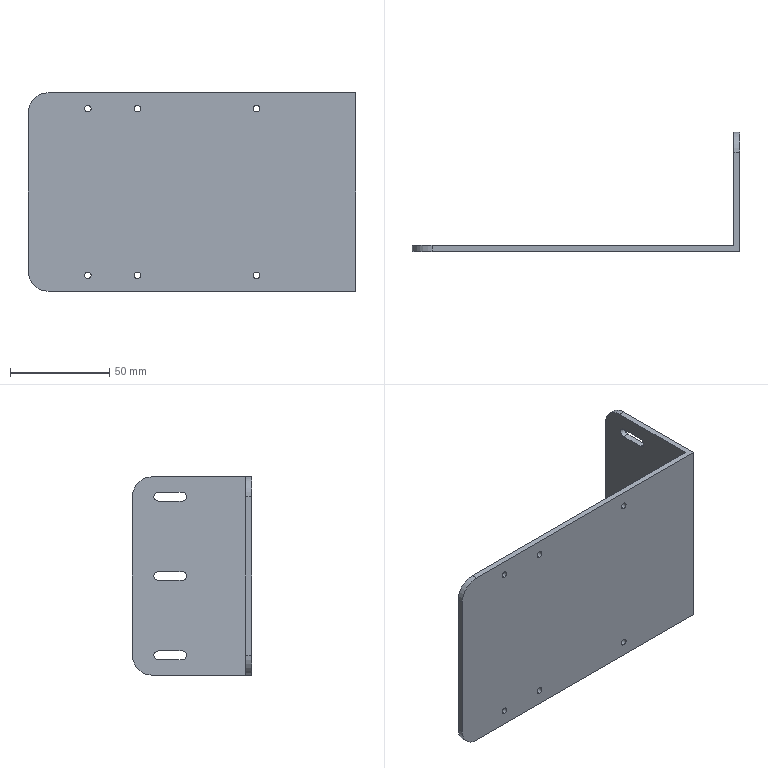Part | NX | features BREP 1 | 1 solid | 36 faces | box 165 x 60 x 100 mm | volume 65559 mm3 | cylinder 22 | plane 14 | commonest cylinder face diameters 3.3 x12 4.5 x6 20 x4
STEP:
#1=CARTESIAN_POINT('',(24.121,-11.746,93.65));
#2=VERTEX_POINT('',#1);
#3=CARTESIAN_POINT('',(24.121,-11.746,90.35));
#4=VERTEX_POINT('',#3);
#5=CARTESIAN_POINT('',(24.121,-11.746,92.));
#6=DIRECTION('',(0.,-1.,0.));
#7=DIRECTION('',(0.,0.,-1.));
#8=AXIS2_PLACEMENT_3D('',#5,#6,#7);
#9=CIRCLE('',#8,1.65);
#10=EDGE_CURVE('',#2,#4,#9,.T.);
#11=ORIENTED_EDGE('',*,*,#10,.T.);
#12=CARTESIAN_POINT('',(24.121,-8.746,90.35));
#13=VERTEX_POINT('',#12);
#14=CARTESIAN_POINT('',(24.121,-8.746,90.35));
#15=DIRECTION('',(0.,1.,0.));
#16=VECTOR('',#15,1000.);
#17=LINE('',#14,#16);
#18=EDGE_CURVE('',#13,#4,#17,.F.);
#19=ORIENTED_EDGE('',*,*,#18,.F.);
#20=CARTESIAN_POINT('',(24.121,-8.746,93.65));
#21=VERTEX_POINT('',#20);
#22=CARTESIAN_POINT('',(24.121,-8.746,92.));
#23=DIRECTION('',(0.,1.,0.));
#24=DIRECTION('',(0.,0.,1.));
#25=AXIS2_PLACEMENT_3D('',#22,#23,#24);
#26=CIRCLE('',#25,1.65);
#27=EDGE_CURVE('',#13,#21,#26,.T.);
#28=ORIENTED_EDGE('',*,*,#27,.T.);
#29=CARTESIAN_POINT('',(24.121,-8.746,93.65));
#30=DIRECTION('',(0.,1.,0.));
#31=VECTOR('',#30,1000.);
#32=LINE('',#29,#31);
#33=EDGE_CURVE('',#21,#2,#32,.F.);
#34=ORIENTED_EDGE('',*,*,#33,.T.);
#35=EDGE_LOOP('',(#11,#19,#28,#34));
#36=FACE_BOUND('',#35,.T.);
#37=CARTESIAN_POINT('',(24.121,-8.746,92.));
#38=DIRECTION('',(0.,1.,0.));
#39=DIRECTION('',(0.,0.,1.));
#40=AXIS2_PLACEMENT_3D('',#37,#38,#39);
#41=CYLINDRICAL_SURFACE('',#40,1.65);
#42=ADVANCED_FACE('',(#36),#41,.F.);
#43=CARTESIAN_POINT('',(49.121,-11.746,93.65));
#44=VERTEX_POINT('',#43);
#45=CARTESIAN_POINT('',(49.121,-11.746,90.35));
#46=VERTEX_POINT('',#45);
#47=CARTESIAN_POINT('',(49.121,-11.746,92.));
#48=DIRECTION('',(0.,-1.,0.));
#49=DIRECTION('',(0.,0.,-1.));
#50=AXIS2_PLACEMENT_3D('',#47,#48,#49);
#51=CIRCLE('',#50,1.65);
#52=EDGE_CURVE('',#44,#46,#51,.T.);
#53=ORIENTED_EDGE('',*,*,#52,.T.);
#54=CARTESIAN_POINT('',(49.121,-8.746,90.35));
#55=VERTEX_POINT('',#54);
#56=CARTESIAN_POINT('',(49.121,-8.746,90.35));
#57=DIRECTION('',(0.,1.,0.));
#58=VECTOR('',#57,1000.);
#59=LINE('',#56,#58);
#60=EDGE_CURVE('',#55,#46,#59,.F.);
#61=ORIENTED_EDGE('',*,*,#60,.F.);
#62=CARTESIAN_POINT('',(49.121,-8.746,93.65));
#63=VERTEX_POINT('',#62);
#64=CARTESIAN_POINT('',(49.121,-8.746,92.));
#65=DIRECTION('',(0.,1.,0.));
#66=DIRECTION('',(0.,0.,1.));
#67=AXIS2_PLACEMENT_3D('',#64,#65,#66);
#68=CIRCLE('',#67,1.65);
#69=EDGE_CURVE('',#55,#63,#68,.T.);
#70=ORIENTED_EDGE('',*,*,#69,.T.);
#71=CARTESIAN_POINT('',(49.121,-8.746,93.65));
#72=DIRECTION('',(0.,1.,0.));
#73=VECTOR('',#72,1000.);
#74=LINE('',#71,#73);
#75=EDGE_CURVE('',#63,#44,#74,.F.);
#76=ORIENTED_EDGE('',*,*,#75,.T.);
#77=EDGE_LOOP('',(#53,#61,#70,#76));
#78=FACE_BOUND('',#77,.T.);
#79=CARTESIAN_POINT('',(49.121,-8.746,92.));
#80=DIRECTION('',(0.,1.,0.));
#81=DIRECTION('',(0.,0.,1.));
#82=AXIS2_PLACEMENT_3D('',#79,#80,#81);
#83=CYLINDRICAL_SURFACE('',#82,1.65);
#84=ADVANCED_FACE('',(#78),#83,.F.);
#85=CARTESIAN_POINT('',(49.121,-11.746,9.65));
#86=VERTEX_POINT('',#85);
#87=CARTESIAN_POINT('',(49.121,-11.746,6.35));
#88=VERTEX_POINT('',#87);
#89=CARTESIAN_POINT('',(49.121,-11.746,8.));
#90=DIRECTION('',(0.,-1.,0.));
#91=DIRECTION('',(0.,0.,-1.));
#92=AXIS2_PLACEMENT_3D('',#89,#90,#91);
#93=CIRCLE('',#92,1.65);
#94=EDGE_CURVE('',#86,#88,#93,.T.);
#95=ORIENTED_EDGE('',*,*,#94,.T.);
#96=CARTESIAN_POINT('',(49.121,-8.746,6.35));
#97=VERTEX_POINT('',#96);
#98=CARTESIAN_POINT('',(49.121,-8.746,6.35));
#99=DIRECTION('',(0.,1.,0.));
#100=VECTOR('',#99,1000.);
#101=LINE('',#98,#100);
#102=EDGE_CURVE('',#97,#88,#101,.F.);
#103=ORIENTED_EDGE('',*,*,#102,.F.);
#104=CARTESIAN_POINT('',(49.121,-8.746,9.65));
#105=VERTEX_POINT('',#104);
#106=CARTESIAN_POINT('',(49.121,-8.746,8.));
#107=DIRECTION('',(0.,1.,0.));
#108=DIRECTION('',(0.,0.,1.));
#109=AXIS2_PLACEMENT_3D('',#106,#107,#108);
#110=CIRCLE('',#109,1.65);
#111=EDGE_CURVE('',#97,#105,#110,.T.);
#112=ORIENTED_EDGE('',*,*,#111,.T.);
#113=CARTESIAN_POINT('',(49.121,-8.746,9.65));
#114=DIRECTION('',(0.,1.,0.));
#115=VECTOR('',#114,1000.);
#116=LINE('',#113,#115);
#117=EDGE_CURVE('',#105,#86,#116,.F.);
#118=ORIENTED_EDGE('',*,*,#117,.T.);
#119=EDGE_LOOP('',(#95,#103,#112,#118));
#120=FACE_BOUND('',#119,.T.);
#121=CARTESIAN_POINT('',(49.121,-8.746,8.));
#122=DIRECTION('',(0.,1.,0.));
#123=DIRECTION('',(0.,0.,1.));
#124=AXIS2_PLACEMENT_3D('',#121,#122,#123);
#125=CYLINDRICAL_SURFACE('',#124,1.65);
#126=ADVANCED_FACE('',(#120),#125,.F.);
#127=CARTESIAN_POINT('',(24.121,-11.746,9.65));
#128=VERTEX_POINT('',#127);
#129=CARTESIAN_POINT('',(24.121,-11.746,6.35));
#130=VERTEX_POINT('',#129);
#131=CARTESIAN_POINT('',(24.121,-11.746,8.));
#132=DIRECTION('',(0.,-1.,0.));
#133=DIRECTION('',(0.,0.,-1.));
#134=AXIS2_PLACEMENT_3D('',#131,#132,#133);
#135=CIRCLE('',#134,1.65);
#136=EDGE_CURVE('',#128,#130,#135,.T.);
#137=ORIENTED_EDGE('',*,*,#136,.T.);
#138=CARTESIAN_POINT('',(24.121,-8.746,6.35));
#139=VERTEX_POINT('',#138);
#140=CARTESIAN_POINT('',(24.121,-8.746,6.35));
#141=DIRECTION('',(0.,1.,0.));
#142=VECTOR('',#141,1000.);
#143=LINE('',#140,#142);
#144=EDGE_CURVE('',#139,#130,#143,.F.);
#145=ORIENTED_EDGE('',*,*,#144,.F.);
#146=CARTESIAN_POINT('',(24.121,-8.746,9.65));
#147=VERTEX_POINT('',#146);
#148=CARTESIAN_POINT('',(24.121,-8.746,8.));
#149=DIRECTION('',(0.,1.,0.));
#150=DIRECTION('',(0.,0.,1.));
#151=AXIS2_PLACEMENT_3D('',#148,#149,#150);
#152=CIRCLE('',#151,1.65);
#153=EDGE_CURVE('',#139,#147,#152,.T.);
#154=ORIENTED_EDGE('',*,*,#153,.T.);
#155=CARTESIAN_POINT('',(24.121,-8.746,9.65));
#156=DIRECTION('',(0.,1.,0.));
#157=VECTOR('',#156,1000.);
#158=LINE('',#155,#157);
#159=EDGE_CURVE('',#147,#128,#158,.F.);
#160=ORIENTED_EDGE('',*,*,#159,.T.);
#161=EDGE_LOOP('',(#137,#145,#154,#160));
#162=FACE_BOUND('',#161,.T.);
#163=CARTESIAN_POINT('',(24.121,-8.746,8.));
#164=DIRECTION('',(0.,1.,0.));
#165=DIRECTION('',(0.,0.,1.));
#166=AXIS2_PLACEMENT_3D('',#163,#164,#165);
#167=CYLINDRICAL_SURFACE('',#166,1.65);
#168=ADVANCED_FACE('',(#162),#167,.F.);
#169=CARTESIAN_POINT('',(109.121,-11.746,9.65));
#170=VERTEX_POINT('',#169);
#171=CARTESIAN_POINT('',(109.121,-11.746,6.35));
#172=VERTEX_POINT('',#171);
#173=CARTESIAN_POINT('',(109.121,-11.746,8.));
#174=DIRECTION('',(0.,-1.,0.));
#175=DIRECTION('',(0.,0.,-1.));
#176=AXIS2_PLACEMENT_3D('',#173,#174,#175);
#177=CIRCLE('',#176,1.65);
#178=EDGE_CURVE('',#170,#172,#177,.T.);
#179=ORIENTED_EDGE('',*,*,#178,.T.);
#180=CARTESIAN_POINT('',(109.121,-8.746,6.35));
#181=VERTEX_POINT('',#180);
#182=CARTESIAN_POINT('',(109.121,-8.746,6.35));
#183=DIRECTION('',(0.,1.,0.));
#184=VECTOR('',#183,1000.);
#185=LINE('',#182,#184);
#186=EDGE_CURVE('',#181,#172,#185,.F.);
#187=ORIENTED_EDGE('',*,*,#186,.F.);
#188=CARTESIAN_POINT('',(109.121,-8.746,9.65));
#189=VERTEX_POINT('',#188);
#190=CARTESIAN_POINT('',(109.121,-8.746,8.));
#191=DIRECTION('',(0.,1.,0.));
#192=DIRECTION('',(0.,0.,1.));
#193=AXIS2_PLACEMENT_3D('',#190,#191,#192);
#194=CIRCLE('',#193,1.65);
#195=EDGE_CURVE('',#181,#189,#194,.T.);
#196=ORIENTED_EDGE('',*,*,#195,.T.);
#197=CARTESIAN_POINT('',(109.121,-8.746,9.65));
#198=DIRECTION('',(0.,1.,0.));
#199=VECTOR('',#198,1000.);
#200=LINE('',#197,#199);
#201=EDGE_CURVE('',#189,#170,#200,.F.);
#202=ORIENTED_EDGE('',*,*,#201,.T.);
#203=EDGE_LOOP('',(#179,#187,#196,#202));
#204=FACE_BOUND('',#203,.T.);
#205=CARTESIAN_POINT('',(109.121,-8.746,8.));
#206=DIRECTION('',(0.,1.,0.));
#207=DIRECTION('',(0.,0.,1.));
#208=AXIS2_PLACEMENT_3D('',#205,#206,#207);
#209=CYLINDRICAL_SURFACE('',#208,1.65);
#210=ADVANCED_FACE('',(#204),#209,.F.);
#211=CARTESIAN_POINT('',(109.121,-11.746,93.65));
#212=VERTEX_POINT('',#211);
#213=CARTESIAN_POINT('',(109.121,-11.746,90.35));
#214=VERTEX_POINT('',#213);
#215=CARTESIAN_POINT('',(109.121,-11.746,92.));
#216=DIRECTION('',(0.,-1.,0.));
#217=DIRECTION('',(0.,0.,-1.));
#218=AXIS2_PLACEMENT_3D('',#215,#216,#217);
#219=CIRCLE('',#218,1.65);
#220=EDGE_CURVE('',#212,#214,#219,.T.);
#221=ORIENTED_EDGE('',*,*,#220,.T.);
#222=CARTESIAN_POINT('',(109.121,-8.746,90.35));
#223=VERTEX_POINT('',#222);
#224=CARTESIAN_POINT('',(109.121,-8.746,90.35));
#225=DIRECTION('',(0.,1.,0.));
#226=VECTOR('',#225,1000.);
#227=LINE('',#224,#226);
#228=EDGE_CURVE('',#223,#214,#227,.F.);
#229=ORIENTED_EDGE('',*,*,#228,.F.);
#230=CARTESIAN_POINT('',(109.121,-8.746,93.65));
#231=VERTEX_POINT('',#230);
#232=CARTESIAN_POINT('',(109.121,-8.746,92.));
#233=DIRECTION('',(0.,1.,0.));
#234=DIRECTION('',(0.,0.,1.));
#235=AXIS2_PLACEMENT_3D('',#232,#233,#234);
#236=CIRCLE('',#235,1.65);
#237=EDGE_CURVE('',#223,#231,#236,.T.);
#238=ORIENTED_EDGE('',*,*,#237,.T.);
#239=CARTESIAN_POINT('',(109.121,-8.746,93.65));
#240=DIRECTION('',(0.,1.,0.));
#241=VECTOR('',#240,1000.);
#242=LINE('',#239,#241);
#243=EDGE_CURVE('',#231,#212,#242,.F.);
#244=ORIENTED_EDGE('',*,*,#243,.T.);
#245=EDGE_LOOP('',(#221,#229,#238,#244));
#246=FACE_BOUND('',#245,.T.);
#247=CARTESIAN_POINT('',(109.121,-8.746,92.));
#248=DIRECTION('',(0.,1.,0.));
#249=DIRECTION('',(0.,0.,1.));
#250=AXIS2_PLACEMENT_3D('',#247,#248,#249);
#251=CYLINDRICAL_SURFACE('',#250,1.65);
#252=ADVANCED_FACE('',(#246),#251,.F.);
#253=CARTESIAN_POINT('',(-5.879,-8.746,90.));
#254=VERTEX_POINT('',#253);
#255=CARTESIAN_POINT('',(-5.879,-8.746,10.));
#256=VERTEX_POINT('',#255);
#257=CARTESIAN_POINT('',(-5.879,-8.746,100.));
#258=DIRECTION('',(0.,0.,-1.));
#259=VECTOR('',#258,1000.);
#260=LINE('',#257,#259);
#261=EDGE_CURVE('',#254,#256,#260,.T.);
#262=ORIENTED_EDGE('',*,*,#261,.F.);
#263=CARTESIAN_POINT('',(4.121,-8.746,100.));
#264=VERTEX_POINT('',#263);
#265=CARTESIAN_POINT('',(4.121,-8.746,90.));
#266=DIRECTION('',(0.,1.,0.));
#267=DIRECTION('',(0.,0.,-1.));
#268=AXIS2_PLACEMENT_3D('',#265,#266,#267);
#269=CIRCLE('',#268,10.);
#270=EDGE_CURVE('',#254,#264,#269,.T.);
#271=ORIENTED_EDGE('',*,*,#270,.T.);
#272=CARTESIAN_POINT('',(156.121,-8.746,100.));
#273=VERTEX_POINT('',#272);
#274=CARTESIAN_POINT('',(159.121,-8.746,100.));
#275=DIRECTION('',(-1.,0.,0.));
#276=VECTOR('',#275,1000.);
#277=LINE('',#274,#276);
#278=EDGE_CURVE('',#273,#264,#277,.T.);
#279=ORIENTED_EDGE('',*,*,#278,.F.);
#280=CARTESIAN_POINT('',(156.121,-8.746,0.));
#281=VERTEX_POINT('',#280);
#282=CARTESIAN_POINT('',(156.121,-8.746,100.));
#283=DIRECTION('',(0.,0.,-1.));
#284=VECTOR('',#283,1000.);
#285=LINE('',#282,#284);
#286=EDGE_CURVE('',#273,#281,#285,.T.);
#287=ORIENTED_EDGE('',*,*,#286,.T.);
#288=CARTESIAN_POINT('',(4.121,-8.746,0.));
#289=VERTEX_POINT('',#288);
#290=CARTESIAN_POINT('',(159.121,-8.746,0.));
#291=DIRECTION('',(-1.,0.,0.));
#292=VECTOR('',#291,1000.);
#293=LINE('',#290,#292);
#294=EDGE_CURVE('',#281,#289,#293,.T.);
#295=ORIENTED_EDGE('',*,*,#294,.T.);
#296=CARTESIAN_POINT('',(4.121,-8.746,10.));
#297=DIRECTION('',(0.,1.,0.));
#298=DIRECTION('',(0.,0.,-1.));
#299=AXIS2_PLACEMENT_3D('',#296,#297,#298);
#300=CIRCLE('',#299,10.);
#301=EDGE_CURVE('',#289,#256,#300,.T.);
#302=ORIENTED_EDGE('',*,*,#301,.T.);
#303=EDGE_LOOP('',(#262,#271,#279,#287,#295,#302));
#304=FACE_BOUND('',#303,.T.);
#305=CARTESIAN_POINT('',(24.121,-8.746,92.));
#306=DIRECTION('',(0.,1.,0.));
#307=DIRECTION('',(0.,0.,1.));
#308=AXIS2_PLACEMENT_3D('',#305,#306,#307);
#309=CIRCLE('',#308,1.65);
#310=EDGE_CURVE('',#21,#13,#309,.T.);
#311=ORIENTED_EDGE('',*,*,#310,.F.);
#312=ORIENTED_EDGE('',*,*,#27,.F.);
#313=EDGE_LOOP('',(#311,#312));
#314=FACE_BOUND('',#313,.T.);
#315=CARTESIAN_POINT('',(49.121,-8.746,92.));
#316=DIRECTION('',(0.,1.,0.));
#317=DIRECTION('',(0.,0.,1.));
#318=AXIS2_PLACEMENT_3D('',#315,#316,#317);
#319=CIRCLE('',#318,1.65);
#320=EDGE_CURVE('',#63,#55,#319,.T.);
#321=ORIENTED_EDGE('',*,*,#320,.F.);
#322=ORIENTED_EDGE('',*,*,#69,.F.);
#323=EDGE_LOOP('',(#321,#322));
#324=FACE_BOUND('',#323,.T.);
#325=CARTESIAN_POINT('',(49.121,-8.746,8.));
#326=DIRECTION('',(0.,1.,0.));
#327=DIRECTION('',(0.,0.,1.));
#328=AXIS2_PLACEMENT_3D('',#325,#326,#327);
#329=CIRCLE('',#328,1.65);
#330=EDGE_CURVE('',#105,#97,#329,.T.);
#331=ORIENTED_EDGE('',*,*,#330,.F.);
#332=ORIENTED_EDGE('',*,*,#111,.F.);
#333=EDGE_LOOP('',(#331,#332));
#334=FACE_BOUND('',#333,.T.);
#335=CARTESIAN_POINT('',(24.121,-8.746,8.));
#336=DIRECTION('',(0.,1.,0.));
#337=DIRECTION('',(0.,0.,1.));
#338=AXIS2_PLACEMENT_3D('',#335,#336,#337);
#339=CIRCLE('',#338,1.65);
#340=EDGE_CURVE('',#147,#139,#339,.T.);
#341=ORIENTED_EDGE('',*,*,#340,.F.);
#342=ORIENTED_EDGE('',*,*,#153,.F.);
#343=EDGE_LOOP('',(#341,#342));
#344=FACE_BOUND('',#343,.T.);
#345=CARTESIAN_POINT('',(109.121,-8.746,8.));
#346=DIRECTION('',(0.,1.,0.));
#347=DIRECTION('',(0.,0.,1.));
#348=AXIS2_PLACEMENT_3D('',#345,#346,#347);
#349=CIRCLE('',#348,1.65);
#350=EDGE_CURVE('',#189,#181,#349,.T.);
#351=ORIENTED_EDGE('',*,*,#350,.F.);
#352=ORIENTED_EDGE('',*,*,#195,.F.);
#353=EDGE_LOOP('',(#351,#352));
#354=FACE_BOUND('',#353,.T.);
#355=CARTESIAN_POINT('',(109.121,-8.746,92.));
#356=DIRECTION('',(0.,1.,0.));
#357=DIRECTION('',(0.,0.,1.));
#358=AXIS2_PLACEMENT_3D('',#355,#356,#357);
#359=CIRCLE('',#358,1.65);
#360=EDGE_CURVE('',#231,#223,#359,.T.);
#361=ORIENTED_EDGE('',*,*,#360,.F.);
#362=ORIENTED_EDGE('',*,*,#237,.F.);
#363=EDGE_LOOP('',(#361,#362));
#364=FACE_BOUND('',#363,.T.);
#365=CARTESIAN_POINT('',(159.121,-8.746,100.));
#366=DIRECTION('',(0.,-1.,0.));
#367=DIRECTION('',(0.,0.,-1.));
#368=AXIS2_PLACEMENT_3D('',#365,#366,#367);
#369=PLANE('',#368);
#370=ADVANCED_FACE('',(#304,#314,#324,#334,#344,#354,#364),#369,.F.);
#371=CARTESIAN_POINT('',(-5.879,-11.746,90.));
#372=VERTEX_POINT('',#371);
#373=CARTESIAN_POINT('',(-5.879,-11.746,10.));
#374=VERTEX_POINT('',#373);
#375=CARTESIAN_POINT('',(-5.879,-11.746,100.));
#376=DIRECTION('',(0.,0.,-1.));
#377=VECTOR('',#376,1000.);
#378=LINE('',#375,#377);
#379=EDGE_CURVE('',#372,#374,#378,.T.);
#380=ORIENTED_EDGE('',*,*,#379,.F.);
#381=CARTESIAN_POINT('',(-5.879,-11.746,90.));
#382=DIRECTION('',(0.,1.,0.));
#383=VECTOR('',#382,1000.);
#384=LINE('',#381,#383);
#385=EDGE_CURVE('',#372,#254,#384,.T.);
#386=ORIENTED_EDGE('',*,*,#385,.T.);
#387=ORIENTED_EDGE('',*,*,#261,.T.);
#388=CARTESIAN_POINT('',(-5.879,-11.746,10.));
#389=DIRECTION('',(0.,-1.,0.));
#390=VECTOR('',#389,1000.);
#391=LINE('',#388,#390);
#392=EDGE_CURVE('',#256,#374,#391,.T.);
#393=ORIENTED_EDGE('',*,*,#392,.T.);
#394=EDGE_LOOP('',(#380,#386,#387,#393));
#395=FACE_BOUND('',#394,.T.);
#396=CARTESIAN_POINT('',(-5.879,-11.746,100.));
#397=DIRECTION('',(-1.,0.,0.));
#398=DIRECTION('',(0.,0.,1.));
#399=AXIS2_PLACEMENT_3D('',#396,#397,#398);
#400=PLANE('',#399);
#401=ADVANCED_FACE('',(#395),#400,.T.);
#402=CARTESIAN_POINT('',(159.121,-11.746,100.));
#403=VERTEX_POINT('',#402);
#404=CARTESIAN_POINT('',(4.121,-11.746,100.));
#405=VERTEX_POINT('',#404);
#406=CARTESIAN_POINT('',(159.121,-11.746,100.));
#407=DIRECTION('',(-1.,0.,0.));
#408=VECTOR('',#407,1000.);
#409=LINE('',#406,#408);
#410=EDGE_CURVE('',#403,#405,#409,.T.);
#411=ORIENTED_EDGE('',*,*,#410,.T.);
#412=CARTESIAN_POINT('',(4.121,-11.746,90.));
#413=DIRECTION('',(0.,-1.,0.));
#414=DIRECTION('',(0.,0.,-1.));
#415=AXIS2_PLACEMENT_3D('',#412,#413,#414);
#416=CIRCLE('',#415,10.);
#417=EDGE_CURVE('',#405,#372,#416,.T.);
#418=ORIENTED_EDGE('',*,*,#417,.T.);
#419=ORIENTED_EDGE('',*,*,#379,.T.);
#420=CARTESIAN_POINT('',(4.121,-11.746,0.));
#421=VERTEX_POINT('',#420);
#422=CARTESIAN_POINT('',(4.121,-11.746,10.));
#423=DIRECTION('',(0.,-1.,0.));
#424=DIRECTION('',(0.,0.,-1.));
#425=AXIS2_PLACEMENT_3D('',#422,#423,#424);
#426=CIRCLE('',#425,10.);
#427=EDGE_CURVE('',#374,#421,#426,.T.);
#428=ORIENTED_EDGE('',*,*,#427,.T.);
#429=CARTESIAN_POINT('',(159.121,-11.746,0.));
#430=VERTEX_POINT('',#429);
#431=CARTESIAN_POINT('',(159.121,-11.746,0.));
#432=DIRECTION('',(-1.,0.,0.));
#433=VECTOR('',#432,1000.);
#434=LINE('',#431,#433);
#435=EDGE_CURVE('',#430,#421,#434,.T.);
#436=ORIENTED_EDGE('',*,*,#435,.F.);
#437=CARTESIAN_POINT('',(159.121,-11.746,100.));
#438=DIRECTION('',(0.,0.,-1.));
#439=VECTOR('',#438,1000.);
#440=LINE('',#437,#439);
#441=EDGE_CURVE('',#403,#430,#440,.T.);
#442=ORIENTED_EDGE('',*,*,#441,.F.);
#443=EDGE_LOOP('',(#411,#418,#419,#428,#436,#442));
#444=FACE_BOUND('',#443,.T.);
#445=ORIENTED_EDGE('',*,*,#10,.F.);
#446=CARTESIAN_POINT('',(24.121,-11.746,92.));
#447=DIRECTION('',(0.,-1.,0.));
#448=DIRECTION('',(0.,0.,-1.));
#449=AXIS2_PLACEMENT_3D('',#446,#447,#448);
#450=CIRCLE('',#449,1.65);
#451=EDGE_CURVE('',#4,#2,#450,.T.);
#452=ORIENTED_EDGE('',*,*,#451,.F.);
#453=EDGE_LOOP('',(#445,#452));
#454=FACE_BOUND('',#453,.T.);
#455=ORIENTED_EDGE('',*,*,#52,.F.);
#456=CARTESIAN_POINT('',(49.121,-11.746,92.));
#457=DIRECTION('',(0.,-1.,0.));
#458=DIRECTION('',(0.,0.,-1.));
#459=AXIS2_PLACEMENT_3D('',#456,#457,#458);
#460=CIRCLE('',#459,1.65);
#461=EDGE_CURVE('',#46,#44,#460,.T.);
#462=ORIENTED_EDGE('',*,*,#461,.F.);
#463=EDGE_LOOP('',(#455,#462));
#464=FACE_BOUND('',#463,.T.);
#465=ORIENTED_EDGE('',*,*,#94,.F.);
#466=CARTESIAN_POINT('',(49.121,-11.746,8.));
#467=DIRECTION('',(0.,-1.,0.));
#468=DIRECTION('',(0.,0.,-1.));
#469=AXIS2_PLACEMENT_3D('',#466,#467,#468);
#470=CIRCLE('',#469,1.65);
#471=EDGE_CURVE('',#88,#86,#470,.T.);
#472=ORIENTED_EDGE('',*,*,#471,.F.);
#473=EDGE_LOOP('',(#465,#472));
#474=FACE_BOUND('',#473,.T.);
#475=ORIENTED_EDGE('',*,*,#136,.F.);
#476=CARTESIAN_POINT('',(24.121,-11.746,8.));
#477=DIRECTION('',(0.,-1.,0.));
#478=DIRECTION('',(0.,0.,-1.));
#479=AXIS2_PLACEMENT_3D('',#476,#477,#478);
#480=CIRCLE('',#479,1.65);
#481=EDGE_CURVE('',#130,#128,#480,.T.);
#482=ORIENTED_EDGE('',*,*,#481,.F.);
#483=EDGE_LOOP('',(#475,#482));
#484=FACE_BOUND('',#483,.T.);
#485=ORIENTED_EDGE('',*,*,#178,.F.);
#486=CARTESIAN_POINT('',(109.121,-11.746,8.));
#487=DIRECTION('',(0.,-1.,0.));
#488=DIRECTION('',(0.,0.,-1.));
#489=AXIS2_PLACEMENT_3D('',#486,#487,#488);
#490=CIRCLE('',#489,1.65);
#491=EDGE_CURVE('',#172,#170,#490,.T.);
#492=ORIENTED_EDGE('',*,*,#491,.F.);
#493=EDGE_LOOP('',(#485,#492));
#494=FACE_BOUND('',#493,.T.);
#495=ORIENTED_EDGE('',*,*,#220,.F.);
#496=CARTESIAN_POINT('',(109.121,-11.746,92.));
#497=DIRECTION('',(0.,-1.,0.));
#498=DIRECTION('',(0.,0.,-1.));
#499=AXIS2_PLACEMENT_3D('',#496,#497,#498);
#500=CIRCLE('',#499,1.65);
#501=EDGE_CURVE('',#214,#212,#500,.T.);
#502=ORIENTED_EDGE('',*,*,#501,.F.);
#503=EDGE_LOOP('',(#495,#502));
#504=FACE_BOUND('',#503,.T.);
#505=CARTESIAN_POINT('',(159.121,-11.746,100.));
#506=DIRECTION('',(0.,-1.,0.));
#507=DIRECTION('',(0.,0.,-1.));
#508=AXIS2_PLACEMENT_3D('',#505,#506,#507);
#509=PLANE('',#508);
#510=ADVANCED_FACE('',(#444,#454,#464,#474,#484,#494,#504),#509,.T.);
#511=CARTESIAN_POINT('',(159.121,38.254,0.));
#512=VERTEX_POINT('',#511);
#513=CARTESIAN_POINT('',(159.121,48.254,0.));
#514=DIRECTION('',(0.,-1.,0.));
#515=VECTOR('',#514,1000.);
#516=LINE('',#513,#515);
#517=EDGE_CURVE('',#512,#430,#516,.T.);
#518=ORIENTED_EDGE('',*,*,#517,.F.);
#519=CARTESIAN_POINT('',(159.121,48.254,10.));
#520=VERTEX_POINT('',#519);
#521=CARTESIAN_POINT('',(159.121,38.254,10.));
#522=DIRECTION('',(1.,0.,0.));
#523=DIRECTION('',(0.,0.,-1.));
#524=AXIS2_PLACEMENT_3D('',#521,#522,#523);
#525=CIRCLE('',#524,10.);
#526=EDGE_CURVE('',#512,#520,#525,.T.);
#527=ORIENTED_EDGE('',*,*,#526,.T.);
#528=CARTESIAN_POINT('',(159.121,48.254,90.));
#529=VERTEX_POINT('',#528);
#530=CARTESIAN_POINT('',(159.121,48.254,100.));
#531=DIRECTION('',(0.,0.,-1.));
#532=VECTOR('',#531,1000.);
#533=LINE('',#530,#532);
#534=EDGE_CURVE('',#529,#520,#533,.T.);
#535=ORIENTED_EDGE('',*,*,#534,.F.);
#536=CARTESIAN_POINT('',(159.121,38.254,100.));
#537=VERTEX_POINT('',#536);
#538=CARTESIAN_POINT('',(159.121,38.254,90.));
#539=DIRECTION('',(1.,0.,0.));
#540=DIRECTION('',(0.,0.,-1.));
#541=AXIS2_PLACEMENT_3D('',#538,#539,#540);
#542=CIRCLE('',#541,10.);
#543=EDGE_CURVE('',#529,#537,#542,.T.);
#544=ORIENTED_EDGE('',*,*,#543,.T.);
#545=CARTESIAN_POINT('',(159.121,48.254,100.));
#546=DIRECTION('',(0.,-1.,0.));
#547=VECTOR('',#546,1000.);
#548=LINE('',#545,#547);
#549=EDGE_CURVE('',#537,#403,#548,.T.);
#550=ORIENTED_EDGE('',*,*,#549,.T.);
#551=ORIENTED_EDGE('',*,*,#441,.T.);
#552=EDGE_LOOP('',(#518,#527,#535,#544,#550,#551));
#553=FACE_BOUND('',#552,.T.);
#554=CARTESIAN_POINT('',(159.121,23.254,92.25));
#555=VERTEX_POINT('',#554);
#556=CARTESIAN_POINT('',(159.121,23.254,87.75));
#557=VERTEX_POINT('',#556);
#558=CARTESIAN_POINT('',(159.121,23.254,90.));
#559=DIRECTION('',(1.,0.,0.));
#560=DIRECTION('',(0.,0.,-1.));
#561=AXIS2_PLACEMENT_3D('',#558,#559,#560);
#562=CIRCLE('',#561,2.25);
#563=EDGE_CURVE('',#555,#557,#562,.T.);
#564=ORIENTED_EDGE('',*,*,#563,.F.);
#565=CARTESIAN_POINT('',(159.121,35.254,92.25));
#566=VERTEX_POINT('',#565);
#567=CARTESIAN_POINT('',(159.121,48.254,92.25));
#568=DIRECTION('',(0.,-1.,0.));
#569=VECTOR('',#568,1000.);
#570=LINE('',#567,#569);
#571=EDGE_CURVE('',#566,#555,#570,.T.);
#572=ORIENTED_EDGE('',*,*,#571,.F.);
#573=CARTESIAN_POINT('',(159.121,35.254,87.75));
#574=VERTEX_POINT('',#573);
#575=CARTESIAN_POINT('',(159.121,35.254,90.));
#576=DIRECTION('',(1.,0.,0.));
#577=DIRECTION('',(0.,0.,-1.));
#578=AXIS2_PLACEMENT_3D('',#575,#576,#577);
#579=CIRCLE('',#578,2.25);
#580=EDGE_CURVE('',#574,#566,#579,.T.);
#581=ORIENTED_EDGE('',*,*,#580,.F.);
#582=CARTESIAN_POINT('',(159.121,48.254,87.75));
#583=DIRECTION('',(0.,1.,0.));
#584=VECTOR('',#583,1000.);
#585=LINE('',#582,#584);
#586=EDGE_CURVE('',#557,#574,#585,.T.);
#587=ORIENTED_EDGE('',*,*,#586,.F.);
#588=EDGE_LOOP('',(#564,#572,#581,#587));
#589=FACE_BOUND('',#588,.T.);
#590=CARTESIAN_POINT('',(159.121,23.254,12.25));
#591=VERTEX_POINT('',#590);
#592=CARTESIAN_POINT('',(159.121,23.254,7.75));
#593=VERTEX_POINT('',#592);
#594=CARTESIAN_POINT('',(159.121,23.254,10.));
#595=DIRECTION('',(1.,0.,0.));
#596=DIRECTION('',(0.,0.,-1.));
#597=AXIS2_PLACEMENT_3D('',#594,#595,#596);
#598=CIRCLE('',#597,2.25);
#599=EDGE_CURVE('',#591,#593,#598,.T.);
#600=ORIENTED_EDGE('',*,*,#599,.F.);
#601=CARTESIAN_POINT('',(159.121,35.254,12.25));
#602=VERTEX_POINT('',#601);
#603=CARTESIAN_POINT('',(159.121,48.254,12.25));
#604=DIRECTION('',(0.,-1.,0.));
#605=VECTOR('',#604,1000.);
#606=LINE('',#603,#605);
#607=EDGE_CURVE('',#602,#591,#606,.T.);
#608=ORIENTED_EDGE('',*,*,#607,.F.);
#609=CARTESIAN_POINT('',(159.121,35.254,7.75));
#610=VERTEX_POINT('',#609);
#611=CARTESIAN_POINT('',(159.121,35.254,10.));
#612=DIRECTION('',(1.,0.,0.));
#613=DIRECTION('',(0.,0.,-1.));
#614=AXIS2_PLACEMENT_3D('',#611,#612,#613);
#615=CIRCLE('',#614,2.25);
#616=EDGE_CURVE('',#610,#602,#615,.T.);
#617=ORIENTED_EDGE('',*,*,#616,.F.);
#618=CARTESIAN_POINT('',(159.121,48.254,7.75));
#619=DIRECTION('',(0.,1.,0.));
#620=VECTOR('',#619,1000.);
#621=LINE('',#618,#620);
#622=EDGE_CURVE('',#593,#610,#621,.T.);
#623=ORIENTED_EDGE('',*,*,#622,.F.);
#624=EDGE_LOOP('',(#600,#608,#617,#623));
#625=FACE_BOUND('',#624,.T.);
#626=CARTESIAN_POINT('',(159.121,23.254,52.25));
#627=VERTEX_POINT('',#626);
#628=CARTESIAN_POINT('',(159.121,23.254,47.75));
#629=VERTEX_POINT('',#628);
#630=CARTESIAN_POINT('',(159.121,23.254,50.));
#631=DIRECTION('',(1.,0.,0.));
#632=DIRECTION('',(0.,0.,-1.));
#633=AXIS2_PLACEMENT_3D('',#630,#631,#632);
#634=CIRCLE('',#633,2.25);
#635=EDGE_CURVE('',#627,#629,#634,.T.);
#636=ORIENTED_EDGE('',*,*,#635,.F.);
#637=CARTESIAN_POINT('',(159.121,35.254,52.25));
#638=VERTEX_POINT('',#637);
#639=CARTESIAN_POINT('',(159.121,48.254,52.25));
#640=DIRECTION('',(0.,-1.,0.));
#641=VECTOR('',#640,1000.);
#642=LINE('',#639,#641);
#643=EDGE_CURVE('',#638,#627,#642,.T.);
#644=ORIENTED_EDGE('',*,*,#643,.F.);
#645=CARTESIAN_POINT('',(159.121,35.254,47.75));
#646=VERTEX_POINT('',#645);
#647=CARTESIAN_POINT('',(159.121,35.254,50.));
#648=DIRECTION('',(1.,0.,0.));
#649=DIRECTION('',(0.,0.,-1.));
#650=AXIS2_PLACEMENT_3D('',#647,#648,#649);
#651=CIRCLE('',#650,2.25);
#652=EDGE_CURVE('',#646,#638,#651,.T.);
#653=ORIENTED_EDGE('',*,*,#652,.F.);
#654=CARTESIAN_POINT('',(159.121,48.254,47.75));
#655=DIRECTION('',(0.,1.,0.));
#656=VECTOR('',#655,1000.);
#657=LINE('',#654,#656);
#658=EDGE_CURVE('',#629,#646,#657,.T.);
#659=ORIENTED_EDGE('',*,*,#658,.F.);
#660=EDGE_LOOP('',(#636,#644,#653,#659));
#661=FACE_BOUND('',#660,.T.);
#662=CARTESIAN_POINT('',(159.121,48.254,100.));
#663=DIRECTION('',(1.,0.,0.));
#664=DIRECTION('',(0.,1.,0.));
#665=AXIS2_PLACEMENT_3D('',#662,#663,#664);
#666=PLANE('',#665);
#667=ADVANCED_FACE('',(#553,#589,#625,#661),#666,.T.);
#668=ORIENTED_EDGE('',*,*,#534,.T.);
#669=CARTESIAN_POINT('',(156.121,48.254,10.));
#670=VERTEX_POINT('',#669);
#671=CARTESIAN_POINT('',(156.121,48.254,10.));
#672=DIRECTION('',(-1.,0.,0.));
#673=VECTOR('',#672,1000.);
#674=LINE('',#671,#673);
#675=EDGE_CURVE('',#520,#670,#674,.T.);
#676=ORIENTED_EDGE('',*,*,#675,.T.);
#677=CARTESIAN_POINT('',(156.121,48.254,90.));
#678=VERTEX_POINT('',#677);
#679=CARTESIAN_POINT('',(156.121,48.254,100.));
#680=DIRECTION('',(0.,0.,-1.));
#681=VECTOR('',#680,1000.);
#682=LINE('',#679,#681);
#683=EDGE_CURVE('',#678,#670,#682,.T.);
#684=ORIENTED_EDGE('',*,*,#683,.F.);
#685=CARTESIAN_POINT('',(156.121,48.254,90.));
#686=DIRECTION('',(1.,0.,0.));
#687=VECTOR('',#686,1000.);
#688=LINE('',#685,#687);
#689=EDGE_CURVE('',#678,#529,#688,.T.);
#690=ORIENTED_EDGE('',*,*,#689,.T.);
#691=EDGE_LOOP('',(#668,#676,#684,#690));
#692=FACE_BOUND('',#691,.T.);
#693=CARTESIAN_POINT('',(156.121,48.254,100.));
#694=DIRECTION('',(0.,1.,0.));
#695=DIRECTION('',(1.,0.,0.));
#696=AXIS2_PLACEMENT_3D('',#693,#694,#695);
#697=PLANE('',#696);
#698=ADVANCED_FACE('',(#692),#697,.T.);
#699=ORIENTED_EDGE('',*,*,#683,.T.);
#700=CARTESIAN_POINT('',(156.121,38.254,0.));
#701=VERTEX_POINT('',#700);
#702=CARTESIAN_POINT('',(156.121,38.254,10.));
#703=DIRECTION('',(-1.,0.,0.));
#704=DIRECTION('',(0.,0.,-1.));
#705=AXIS2_PLACEMENT_3D('',#702,#703,#704);
#706=CIRCLE('',#705,10.);
#707=EDGE_CURVE('',#670,#701,#706,.T.);
#708=ORIENTED_EDGE('',*,*,#707,.T.);
#709=CARTESIAN_POINT('',(156.121,48.254,0.));
#710=DIRECTION('',(0.,-1.,0.));
#711=VECTOR('',#710,1000.);
#712=LINE('',#709,#711);
#713=EDGE_CURVE('',#701,#281,#712,.T.);
#714=ORIENTED_EDGE('',*,*,#713,.T.);
#715=ORIENTED_EDGE('',*,*,#286,.F.);
#716=CARTESIAN_POINT('',(156.121,38.254,100.));
#717=VERTEX_POINT('',#716);
#718=CARTESIAN_POINT('',(156.121,48.254,100.));
#719=DIRECTION('',(0.,-1.,0.));
#720=VECTOR('',#719,1000.);
#721=LINE('',#718,#720);
#722=EDGE_CURVE('',#717,#273,#721,.T.);
#723=ORIENTED_EDGE('',*,*,#722,.F.);
#724=CARTESIAN_POINT('',(156.121,38.254,90.));
#725=DIRECTION('',(-1.,0.,0.));
#726=DIRECTION('',(0.,0.,-1.));
#727=AXIS2_PLACEMENT_3D('',#724,#725,#726);
#728=CIRCLE('',#727,10.);
#729=EDGE_CURVE('',#717,#678,#728,.T.);
#730=ORIENTED_EDGE('',*,*,#729,.T.);
#731=EDGE_LOOP('',(#699,#708,#714,#715,#723,#730));
#732=FACE_BOUND('',#731,.T.);
#733=CARTESIAN_POINT('',(156.121,23.254,92.25));
#734=VERTEX_POINT('',#733);
#735=CARTESIAN_POINT('',(156.121,35.254,92.25));
#736=VERTEX_POINT('',#735);
#737=CARTESIAN_POINT('',(156.121,23.254,92.25));
#738=DIRECTION('',(0.,1.,0.));
#739=VECTOR('',#738,1000.);
#740=LINE('',#737,#739);
#741=EDGE_CURVE('',#734,#736,#740,.T.);
#742=ORIENTED_EDGE('',*,*,#741,.F.);
#743=CARTESIAN_POINT('',(156.121,23.254,87.75));
#744=VERTEX_POINT('',#743);
#745=CARTESIAN_POINT('',(156.121,23.254,90.));
#746=DIRECTION('',(-1.,0.,0.));
#747=DIRECTION('',(0.,0.,-1.));
#748=AXIS2_PLACEMENT_3D('',#745,#746,#747);
#749=CIRCLE('',#748,2.25);
#750=EDGE_CURVE('',#744,#734,#749,.T.);
#751=ORIENTED_EDGE('',*,*,#750,.F.);
#752=CARTESIAN_POINT('',(156.121,35.254,87.75));
#753=VERTEX_POINT('',#752);
#754=CARTESIAN_POINT('',(156.121,23.254,87.75));
#755=DIRECTION('',(0.,-1.,0.));
#756=VECTOR('',#755,1000.);
#757=LINE('',#754,#756);
#758=EDGE_CURVE('',#753,#744,#757,.T.);
#759=ORIENTED_EDGE('',*,*,#758,.F.);
#760=CARTESIAN_POINT('',(156.121,35.254,90.));
#761=DIRECTION('',(-1.,0.,0.));
#762=DIRECTION('',(0.,0.,-1.));
#763=AXIS2_PLACEMENT_3D('',#760,#761,#762);
#764=CIRCLE('',#763,2.25);
#765=EDGE_CURVE('',#736,#753,#764,.T.);
#766=ORIENTED_EDGE('',*,*,#765,.F.);
#767=EDGE_LOOP('',(#742,#751,#759,#766));
#768=FACE_BOUND('',#767,.T.);
#769=CARTESIAN_POINT('',(156.121,23.254,12.25));
#770=VERTEX_POINT('',#769);
#771=CARTESIAN_POINT('',(156.121,35.254,12.25));
#772=VERTEX_POINT('',#771);
#773=CARTESIAN_POINT('',(156.121,23.254,12.25));
#774=DIRECTION('',(0.,1.,0.));
#775=VECTOR('',#774,1000.);
#776=LINE('',#773,#775);
#777=EDGE_CURVE('',#770,#772,#776,.T.);
#778=ORIENTED_EDGE('',*,*,#777,.F.);
#779=CARTESIAN_POINT('',(156.121,23.254,7.75));
#780=VERTEX_POINT('',#779);
#781=CARTESIAN_POINT('',(156.121,23.254,10.));
#782=DIRECTION('',(-1.,0.,0.));
#783=DIRECTION('',(0.,0.,1.));
#784=AXIS2_PLACEMENT_3D('',#781,#782,#783);
#785=CIRCLE('',#784,2.25);
#786=EDGE_CURVE('',#780,#770,#785,.T.);
#787=ORIENTED_EDGE('',*,*,#786,.F.);
#788=CARTESIAN_POINT('',(156.121,35.254,7.75));
#789=VERTEX_POINT('',#788);
#790=CARTESIAN_POINT('',(156.121,23.254,7.75));
#791=DIRECTION('',(0.,-1.,0.));
#792=VECTOR('',#791,1000.);
#793=LINE('',#790,#792);
#794=EDGE_CURVE('',#789,#780,#793,.T.);
#795=ORIENTED_EDGE('',*,*,#794,.F.);
#796=CARTESIAN_POINT('',(156.121,35.254,10.));
#797=DIRECTION('',(-1.,0.,0.));
#798=DIRECTION('',(0.,0.,1.));
#799=AXIS2_PLACEMENT_3D('',#796,#797,#798);
#800=CIRCLE('',#799,2.25);
#801=EDGE_CURVE('',#772,#789,#800,.T.);
#802=ORIENTED_EDGE('',*,*,#801,.F.);
#803=EDGE_LOOP('',(#778,#787,#795,#802));
#804=FACE_BOUND('',#803,.T.);
#805=CARTESIAN_POINT('',(156.121,23.254,52.25));
#806=VERTEX_POINT('',#805);
#807=CARTESIAN_POINT('',(156.121,35.254,52.25));
#808=VERTEX_POINT('',#807);
#809=CARTESIAN_POINT('',(156.121,23.254,52.25));
#810=DIRECTION('',(0.,1.,0.));
#811=VECTOR('',#810,1000.);
#812=LINE('',#809,#811);
#813=EDGE_CURVE('',#806,#808,#812,.T.);
#814=ORIENTED_EDGE('',*,*,#813,.F.);
#815=CARTESIAN_POINT('',(156.121,23.254,47.75));
#816=VERTEX_POINT('',#815);
#817=CARTESIAN_POINT('',(156.121,23.254,50.));
#818=DIRECTION('',(-1.,0.,0.));
#819=DIRECTION('',(0.,0.,1.));
#820=AXIS2_PLACEMENT_3D('',#817,#818,#819);
#821=CIRCLE('',#820,2.25);
#822=EDGE_CURVE('',#816,#806,#821,.T.);
#823=ORIENTED_EDGE('',*,*,#822,.F.);
#824=CARTESIAN_POINT('',(156.121,35.254,47.75));
#825=VERTEX_POINT('',#824);
#826=CARTESIAN_POINT('',(156.121,23.254,47.75));
#827=DIRECTION('',(0.,-1.,0.));
#828=VECTOR('',#827,1000.);
#829=LINE('',#826,#828);
#830=EDGE_CURVE('',#825,#816,#829,.T.);
#831=ORIENTED_EDGE('',*,*,#830,.F.);
#832=CARTESIAN_POINT('',(156.121,35.254,50.));
#833=DIRECTION('',(-1.,0.,0.));
#834=DIRECTION('',(0.,0.,1.));
#835=AXIS2_PLACEMENT_3D('',#832,#833,#834);
#836=CIRCLE('',#835,2.25);
#837=EDGE_CURVE('',#808,#825,#836,.T.);
#838=ORIENTED_EDGE('',*,*,#837,.F.);
#839=EDGE_LOOP('',(#814,#823,#831,#838));
#840=FACE_BOUND('',#839,.T.);
#841=CARTESIAN_POINT('',(156.121,48.254,100.));
#842=DIRECTION('',(1.,0.,0.));
#843=DIRECTION('',(0.,1.,0.));
#844=AXIS2_PLACEMENT_3D('',#841,#842,#843);
#845=PLANE('',#844);
#846=ADVANCED_FACE('',(#732,#768,#804,#840),#845,.F.);
#847=ORIENTED_EDGE('',*,*,#549,.F.);
#848=CARTESIAN_POINT('',(-5.879,38.254,100.));
#849=DIRECTION('',(-1.,0.,0.));
#850=VECTOR('',#849,1000.);
#851=LINE('',#848,#850);
#852=EDGE_CURVE('',#537,#717,#851,.T.);
#853=ORIENTED_EDGE('',*,*,#852,.T.);
#854=ORIENTED_EDGE('',*,*,#722,.T.);
#855=ORIENTED_EDGE('',*,*,#278,.T.);
#856=CARTESIAN_POINT('',(4.121,-8.746,100.));
#857=DIRECTION('',(0.,-1.,0.));
#858=VECTOR('',#857,1000.);
#859=LINE('',#856,#858);
#860=EDGE_CURVE('',#264,#405,#859,.T.);
#861=ORIENTED_EDGE('',*,*,#860,.T.);
#862=ORIENTED_EDGE('',*,*,#410,.F.);
#863=EDGE_LOOP('',(#847,#853,#854,#855,#861,#862));
#864=FACE_BOUND('',#863,.T.);
#865=CARTESIAN_POINT('',(-5.879,-8.746,100.));
#866=DIRECTION('',(0.,0.,1.));
#867=DIRECTION('',(1.,0.,0.));
#868=AXIS2_PLACEMENT_3D('',#865,#866,#867);
#869=PLANE('',#868);
#870=ADVANCED_FACE('',(#864),#869,.T.);
#871=ORIENTED_EDGE('',*,*,#713,.F.);
#872=CARTESIAN_POINT('',(159.121,38.254,0.));
#873=DIRECTION('',(1.,0.,0.));
#874=VECTOR('',#873,1000.);
#875=LINE('',#872,#874);
#876=EDGE_CURVE('',#701,#512,#875,.T.);
#877=ORIENTED_EDGE('',*,*,#876,.T.);
#878=ORIENTED_EDGE('',*,*,#517,.T.);
#879=ORIENTED_EDGE('',*,*,#435,.T.);
#880=CARTESIAN_POINT('',(4.121,-8.746,0.));
#881=DIRECTION('',(0.,1.,0.));
#882=VECTOR('',#881,1000.);
#883=LINE('',#880,#882);
#884=EDGE_CURVE('',#421,#289,#883,.T.);
#885=ORIENTED_EDGE('',*,*,#884,.T.);
#886=ORIENTED_EDGE('',*,*,#294,.F.);
#887=EDGE_LOOP('',(#871,#877,#878,#879,#885,#886));
#888=FACE_BOUND('',#887,.T.);
#889=CARTESIAN_POINT('',(-5.879,-8.746,0.));
#890=DIRECTION('',(0.,0.,1.));
#891=DIRECTION('',(1.,0.,0.));
#892=AXIS2_PLACEMENT_3D('',#889,#890,#891);
#893=PLANE('',#892);
#894=ADVANCED_FACE('',(#888),#893,.F.);
#895=ORIENTED_EDGE('',*,*,#707,.F.);
#896=ORIENTED_EDGE('',*,*,#675,.F.);
#897=ORIENTED_EDGE('',*,*,#526,.F.);
#898=ORIENTED_EDGE('',*,*,#876,.F.);
#899=EDGE_LOOP('',(#895,#896,#897,#898));
#900=FACE_BOUND('',#899,.T.);
#901=CARTESIAN_POINT('',(-5.879,38.254,10.));
#902=DIRECTION('',(-1.,0.,0.));
#903=DIRECTION('',(0.,0.,1.));
#904=AXIS2_PLACEMENT_3D('',#901,#902,#903);
#905=CYLINDRICAL_SURFACE('',#904,10.);
#906=ADVANCED_FACE('',(#900),#905,.T.);
#907=ORIENTED_EDGE('',*,*,#729,.F.);
#908=ORIENTED_EDGE('',*,*,#852,.F.);
#909=ORIENTED_EDGE('',*,*,#543,.F.);
#910=ORIENTED_EDGE('',*,*,#689,.F.);
#911=EDGE_LOOP('',(#907,#908,#909,#910));
#912=FACE_BOUND('',#911,.T.);
#913=CARTESIAN_POINT('',(156.121,38.254,90.));
#914=DIRECTION('',(1.,0.,0.));
#915=DIRECTION('',(0.,0.,-1.));
#916=AXIS2_PLACEMENT_3D('',#913,#914,#915);
#917=CYLINDRICAL_SURFACE('',#916,10.);
#918=ADVANCED_FACE('',(#912),#917,.T.);
#919=ORIENTED_EDGE('',*,*,#417,.F.);
#920=ORIENTED_EDGE('',*,*,#860,.F.);
#921=ORIENTED_EDGE('',*,*,#270,.F.);
#922=ORIENTED_EDGE('',*,*,#385,.F.);
#923=EDGE_LOOP('',(#919,#920,#921,#922));
#924=FACE_BOUND('',#923,.T.);
#925=CARTESIAN_POINT('',(4.121,-11.746,90.));
#926=DIRECTION('',(0.,1.,0.));
#927=DIRECTION('',(0.,0.,1.));
#928=AXIS2_PLACEMENT_3D('',#925,#926,#927);
#929=CYLINDRICAL_SURFACE('',#928,10.);
#930=ADVANCED_FACE('',(#924),#929,.T.);
#931=ORIENTED_EDGE('',*,*,#427,.F.);
#932=ORIENTED_EDGE('',*,*,#392,.F.);
#933=ORIENTED_EDGE('',*,*,#301,.F.);
#934=ORIENTED_EDGE('',*,*,#884,.F.);
#935=EDGE_LOOP('',(#931,#932,#933,#934));
#936=FACE_BOUND('',#935,.T.);
#937=CARTESIAN_POINT('',(4.121,-8.746,10.));
#938=DIRECTION('',(0.,-1.,0.));
#939=DIRECTION('',(0.,0.,-1.));
#940=AXIS2_PLACEMENT_3D('',#937,#938,#939);
#941=CYLINDRICAL_SURFACE('',#940,10.);
#942=ADVANCED_FACE('',(#936),#941,.T.);
#943=ORIENTED_EDGE('',*,*,#228,.T.);
#944=ORIENTED_EDGE('',*,*,#501,.T.);
#945=ORIENTED_EDGE('',*,*,#243,.F.);
#946=ORIENTED_EDGE('',*,*,#360,.T.);
#947=EDGE_LOOP('',(#943,#944,#945,#946));
#948=FACE_BOUND('',#947,.T.);
#949=CARTESIAN_POINT('',(109.121,-8.746,92.));
#950=DIRECTION('',(0.,1.,0.));
#951=DIRECTION('',(0.,0.,1.));
#952=AXIS2_PLACEMENT_3D('',#949,#950,#951);
#953=CYLINDRICAL_SURFACE('',#952,1.65);
#954=ADVANCED_FACE('',(#948),#953,.F.);
#955=ORIENTED_EDGE('',*,*,#186,.T.);
#956=ORIENTED_EDGE('',*,*,#491,.T.);
#957=ORIENTED_EDGE('',*,*,#201,.F.);
#958=ORIENTED_EDGE('',*,*,#350,.T.);
#959=EDGE_LOOP('',(#955,#956,#957,#958));
#960=FACE_BOUND('',#959,.T.);
#961=CARTESIAN_POINT('',(109.121,-8.746,8.));
#962=DIRECTION('',(0.,1.,0.));
#963=DIRECTION('',(0.,0.,1.));
#964=AXIS2_PLACEMENT_3D('',#961,#962,#963);
#965=CYLINDRICAL_SURFACE('',#964,1.65);
#966=ADVANCED_FACE('',(#960),#965,.F.);
#967=ORIENTED_EDGE('',*,*,#144,.T.);
#968=ORIENTED_EDGE('',*,*,#481,.T.);
#969=ORIENTED_EDGE('',*,*,#159,.F.);
#970=ORIENTED_EDGE('',*,*,#340,.T.);
#971=EDGE_LOOP('',(#967,#968,#969,#970));
#972=FACE_BOUND('',#971,.T.);
#973=CARTESIAN_POINT('',(24.121,-8.746,8.));
#974=DIRECTION('',(0.,1.,0.));
#975=DIRECTION('',(0.,0.,1.));
#976=AXIS2_PLACEMENT_3D('',#973,#974,#975);
#977=CYLINDRICAL_SURFACE('',#976,1.65);
#978=ADVANCED_FACE('',(#972),#977,.F.);
#979=ORIENTED_EDGE('',*,*,#102,.T.);
#980=ORIENTED_EDGE('',*,*,#471,.T.);
#981=ORIENTED_EDGE('',*,*,#117,.F.);
#982=ORIENTED_EDGE('',*,*,#330,.T.);
#983=EDGE_LOOP('',(#979,#980,#981,#982));
#984=FACE_BOUND('',#983,.T.);
#985=CARTESIAN_POINT('',(49.121,-8.746,8.));
#986=DIRECTION('',(0.,1.,0.));
#987=DIRECTION('',(0.,0.,1.));
#988=AXIS2_PLACEMENT_3D('',#985,#986,#987);
#989=CYLINDRICAL_SURFACE('',#988,1.65);
#990=ADVANCED_FACE('',(#984),#989,.F.);
#991=ORIENTED_EDGE('',*,*,#60,.T.);
#992=ORIENTED_EDGE('',*,*,#461,.T.);
#993=ORIENTED_EDGE('',*,*,#75,.F.);
#994=ORIENTED_EDGE('',*,*,#320,.T.);
#995=EDGE_LOOP('',(#991,#992,#993,#994));
#996=FACE_BOUND('',#995,.T.);
#997=CARTESIAN_POINT('',(49.121,-8.746,92.));
#998=DIRECTION('',(0.,1.,0.));
#999=DIRECTION('',(0.,0.,1.));
#1000=AXIS2_PLACEMENT_3D('',#997,#998,#999);
#1001=CYLINDRICAL_SURFACE('',#1000,1.65);
#1002=ADVANCED_FACE('',(#996),#1001,.F.);
#1003=ORIENTED_EDGE('',*,*,#18,.T.);
#1004=ORIENTED_EDGE('',*,*,#451,.T.);
#1005=ORIENTED_EDGE('',*,*,#33,.F.);
#1006=ORIENTED_EDGE('',*,*,#310,.T.);
#1007=EDGE_LOOP('',(#1003,#1004,#1005,#1006));
#1008=FACE_BOUND('',#1007,.T.);
#1009=CARTESIAN_POINT('',(24.121,-8.746,92.));
#1010=DIRECTION('',(0.,1.,0.));
#1011=DIRECTION('',(0.,0.,1.));
#1012=AXIS2_PLACEMENT_3D('',#1009,#1010,#1011);
#1013=CYLINDRICAL_SURFACE('',#1012,1.65);
#1014=ADVANCED_FACE('',(#1008),#1013,.F.);
#1015=ORIENTED_EDGE('',*,*,#635,.T.);
#1016=CARTESIAN_POINT('',(166.121,23.254,47.75));
#1017=DIRECTION('',(-1.,0.,0.));
#1018=VECTOR('',#1017,1000.);
#1019=LINE('',#1016,#1018);
#1020=EDGE_CURVE('',#629,#816,#1019,.T.);
#1021=ORIENTED_EDGE('',*,*,#1020,.T.);
#1022=ORIENTED_EDGE('',*,*,#822,.T.);
#1023=CARTESIAN_POINT('',(166.121,23.254,52.25));
#1024=DIRECTION('',(-1.,0.,0.));
#1025=VECTOR('',#1024,1000.);
#1026=LINE('',#1023,#1025);
#1027=EDGE_CURVE('',#627,#806,#1026,.T.);
#1028=ORIENTED_EDGE('',*,*,#1027,.F.);
#1029=EDGE_LOOP('',(#1015,#1021,#1022,#1028));
#1030=FACE_BOUND('',#1029,.T.);
#1031=CARTESIAN_POINT('',(166.121,23.254,50.));
#1032=DIRECTION('',(-1.,0.,0.));
#1033=DIRECTION('',(0.,0.,1.));
#1034=AXIS2_PLACEMENT_3D('',#1031,#1032,#1033);
#1035=CYLINDRICAL_SURFACE('',#1034,2.25);
#1036=ADVANCED_FACE('',(#1030),#1035,.F.);
#1037=ORIENTED_EDGE('',*,*,#658,.T.);
#1038=CARTESIAN_POINT('',(166.121,35.254,47.75));
#1039=DIRECTION('',(-1.,0.,0.));
#1040=VECTOR('',#1039,1000.);
#1041=LINE('',#1038,#1040);
#1042=EDGE_CURVE('',#646,#825,#1041,.T.);
#1043=ORIENTED_EDGE('',*,*,#1042,.T.);
#1044=ORIENTED_EDGE('',*,*,#830,.T.);
#1045=ORIENTED_EDGE('',*,*,#1020,.F.);
#1046=EDGE_LOOP('',(#1037,#1043,#1044,#1045));
#1047=FACE_BOUND('',#1046,.T.);
#1048=CARTESIAN_POINT('',(166.121,23.254,47.75));
#1049=DIRECTION('',(0.,0.,-1.));
#1050=DIRECTION('',(0.,-1.,0.));
#1051=AXIS2_PLACEMENT_3D('',#1048,#1049,#1050);
#1052=PLANE('',#1051);
#1053=ADVANCED_FACE('',(#1047),#1052,.F.);
#1054=ORIENTED_EDGE('',*,*,#652,.T.);
#1055=CARTESIAN_POINT('',(166.121,35.254,52.25));
#1056=DIRECTION('',(-1.,0.,0.));
#1057=VECTOR('',#1056,1000.);
#1058=LINE('',#1055,#1057);
#1059=EDGE_CURVE('',#638,#808,#1058,.T.);
#1060=ORIENTED_EDGE('',*,*,#1059,.T.);
#1061=ORIENTED_EDGE('',*,*,#837,.T.);
#1062=ORIENTED_EDGE('',*,*,#1042,.F.);
#1063=EDGE_LOOP('',(#1054,#1060,#1061,#1062));
#1064=FACE_BOUND('',#1063,.T.);
#1065=CARTESIAN_POINT('',(166.121,35.254,50.));
#1066=DIRECTION('',(-1.,0.,0.));
#1067=DIRECTION('',(0.,0.,1.));
#1068=AXIS2_PLACEMENT_3D('',#1065,#1066,#1067);
#1069=CYLINDRICAL_SURFACE('',#1068,2.25);
#1070=ADVANCED_FACE('',(#1064),#1069,.F.);
#1071=ORIENTED_EDGE('',*,*,#643,.T.);
#1072=ORIENTED_EDGE('',*,*,#1027,.T.);
#1073=ORIENTED_EDGE('',*,*,#813,.T.);
#1074=ORIENTED_EDGE('',*,*,#1059,.F.);
#1075=EDGE_LOOP('',(#1071,#1072,#1073,#1074));
#1076=FACE_BOUND('',#1075,.T.);
#1077=CARTESIAN_POINT('',(166.121,23.254,52.25));
#1078=DIRECTION('',(0.,0.,1.));
#1079=DIRECTION('',(1.,0.,0.));
#1080=AXIS2_PLACEMENT_3D('',#1077,#1078,#1079);
#1081=PLANE('',#1080);
#1082=ADVANCED_FACE('',(#1076),#1081,.F.);
#1083=ORIENTED_EDGE('',*,*,#599,.T.);
#1084=CARTESIAN_POINT('',(166.121,23.254,7.75));
#1085=DIRECTION('',(-1.,0.,0.));
#1086=VECTOR('',#1085,1000.);
#1087=LINE('',#1084,#1086);
#1088=EDGE_CURVE('',#593,#780,#1087,.T.);
#1089=ORIENTED_EDGE('',*,*,#1088,.T.);
#1090=ORIENTED_EDGE('',*,*,#786,.T.);
#1091=CARTESIAN_POINT('',(166.121,23.254,12.25));
#1092=DIRECTION('',(-1.,0.,0.));
#1093=VECTOR('',#1092,1000.);
#1094=LINE('',#1091,#1093);
#1095=EDGE_CURVE('',#591,#770,#1094,.T.);
#1096=ORIENTED_EDGE('',*,*,#1095,.F.);
#1097=EDGE_LOOP('',(#1083,#1089,#1090,#1096));
#1098=FACE_BOUND('',#1097,.T.);
#1099=CARTESIAN_POINT('',(166.121,23.254,10.));
#1100=DIRECTION('',(-1.,0.,0.));
#1101=DIRECTION('',(0.,0.,1.));
#1102=AXIS2_PLACEMENT_3D('',#1099,#1100,#1101);
#1103=CYLINDRICAL_SURFACE('',#1102,2.25);
#1104=ADVANCED_FACE('',(#1098),#1103,.F.);
#1105=ORIENTED_EDGE('',*,*,#622,.T.);
#1106=CARTESIAN_POINT('',(166.121,35.254,7.75));
#1107=DIRECTION('',(-1.,0.,0.));
#1108=VECTOR('',#1107,1000.);
#1109=LINE('',#1106,#1108);
#1110=EDGE_CURVE('',#610,#789,#1109,.T.);
#1111=ORIENTED_EDGE('',*,*,#1110,.T.);
#1112=ORIENTED_EDGE('',*,*,#794,.T.);
#1113=ORIENTED_EDGE('',*,*,#1088,.F.);
#1114=EDGE_LOOP('',(#1105,#1111,#1112,#1113));
#1115=FACE_BOUND('',#1114,.T.);
#1116=CARTESIAN_POINT('',(166.121,23.254,7.75));
#1117=DIRECTION('',(0.,0.,-1.));
#1118=DIRECTION('',(0.,-1.,0.));
#1119=AXIS2_PLACEMENT_3D('',#1116,#1117,#1118);
#1120=PLANE('',#1119);
#1121=ADVANCED_FACE('',(#1115),#1120,.F.);
#1122=ORIENTED_EDGE('',*,*,#616,.T.);
#1123=CARTESIAN_POINT('',(166.121,35.254,12.25));
#1124=DIRECTION('',(-1.,0.,0.));
#1125=VECTOR('',#1124,1000.);
#1126=LINE('',#1123,#1125);
#1127=EDGE_CURVE('',#602,#772,#1126,.T.);
#1128=ORIENTED_EDGE('',*,*,#1127,.T.);
#1129=ORIENTED_EDGE('',*,*,#801,.T.);
#1130=ORIENTED_EDGE('',*,*,#1110,.F.);
#1131=EDGE_LOOP('',(#1122,#1128,#1129,#1130));
#1132=FACE_BOUND('',#1131,.T.);
#1133=CARTESIAN_POINT('',(166.121,35.254,10.));
#1134=DIRECTION('',(-1.,0.,0.));
#1135=DIRECTION('',(0.,0.,1.));
#1136=AXIS2_PLACEMENT_3D('',#1133,#1134,#1135);
#1137=CYLINDRICAL_SURFACE('',#1136,2.25);
#1138=ADVANCED_FACE('',(#1132),#1137,.F.);
#1139=ORIENTED_EDGE('',*,*,#607,.T.);
#1140=ORIENTED_EDGE('',*,*,#1095,.T.);
#1141=ORIENTED_EDGE('',*,*,#777,.T.);
#1142=ORIENTED_EDGE('',*,*,#1127,.F.);
#1143=EDGE_LOOP('',(#1139,#1140,#1141,#1142));
#1144=FACE_BOUND('',#1143,.T.);
#1145=CARTESIAN_POINT('',(166.121,23.254,12.25));
#1146=DIRECTION('',(0.,0.,1.));
#1147=DIRECTION('',(0.,-1.,0.));
#1148=AXIS2_PLACEMENT_3D('',#1145,#1146,#1147);
#1149=PLANE('',#1148);
#1150=ADVANCED_FACE('',(#1144),#1149,.F.);
#1151=ORIENTED_EDGE('',*,*,#563,.T.);
#1152=CARTESIAN_POINT('',(166.121,23.254,87.75));
#1153=DIRECTION('',(-1.,0.,0.));
#1154=VECTOR('',#1153,1000.);
#1155=LINE('',#1152,#1154);
#1156=EDGE_CURVE('',#557,#744,#1155,.T.);
#1157=ORIENTED_EDGE('',*,*,#1156,.T.);
#1158=ORIENTED_EDGE('',*,*,#750,.T.);
#1159=CARTESIAN_POINT('',(166.121,23.254,92.25));
#1160=DIRECTION('',(-1.,0.,0.));
#1161=VECTOR('',#1160,1000.);
#1162=LINE('',#1159,#1161);
#1163=EDGE_CURVE('',#555,#734,#1162,.T.);
#1164=ORIENTED_EDGE('',*,*,#1163,.F.);
#1165=EDGE_LOOP('',(#1151,#1157,#1158,#1164));
#1166=FACE_BOUND('',#1165,.T.);
#1167=CARTESIAN_POINT('',(166.121,23.254,90.));
#1168=DIRECTION('',(-1.,0.,0.));
#1169=DIRECTION('',(0.,0.,1.));
#1170=AXIS2_PLACEMENT_3D('',#1167,#1168,#1169);
#1171=CYLINDRICAL_SURFACE('',#1170,2.25);
#1172=ADVANCED_FACE('',(#1166),#1171,.F.);
#1173=ORIENTED_EDGE('',*,*,#586,.T.);
#1174=CARTESIAN_POINT('',(166.121,35.254,87.75));
#1175=DIRECTION('',(-1.,0.,0.));
#1176=VECTOR('',#1175,1000.);
#1177=LINE('',#1174,#1176);
#1178=EDGE_CURVE('',#574,#753,#1177,.T.);
#1179=ORIENTED_EDGE('',*,*,#1178,.T.);
#1180=ORIENTED_EDGE('',*,*,#758,.T.);
#1181=ORIENTED_EDGE('',*,*,#1156,.F.);
#1182=EDGE_LOOP('',(#1173,#1179,#1180,#1181));
#1183=FACE_BOUND('',#1182,.T.);
#1184=CARTESIAN_POINT('',(166.121,23.254,87.75));
#1185=DIRECTION('',(0.,0.,-1.));
#1186=DIRECTION('',(-1.,0.,0.));
#1187=AXIS2_PLACEMENT_3D('',#1184,#1185,#1186);
#1188=PLANE('',#1187);
#1189=ADVANCED_FACE('',(#1183),#1188,.F.);
#1190=ORIENTED_EDGE('',*,*,#580,.T.);
#1191=CARTESIAN_POINT('',(166.121,35.254,92.25));
#1192=DIRECTION('',(-1.,0.,0.));
#1193=VECTOR('',#1192,1000.);
#1194=LINE('',#1191,#1193);
#1195=EDGE_CURVE('',#566,#736,#1194,.T.);
#1196=ORIENTED_EDGE('',*,*,#1195,.T.);
#1197=ORIENTED_EDGE('',*,*,#765,.T.);
#1198=ORIENTED_EDGE('',*,*,#1178,.F.);
#1199=EDGE_LOOP('',(#1190,#1196,#1197,#1198));
#1200=FACE_BOUND('',#1199,.T.);
#1201=CARTESIAN_POINT('',(166.121,35.254,90.));
#1202=DIRECTION('',(-1.,0.,0.));
#1203=DIRECTION('',(0.,0.,1.));
#1204=AXIS2_PLACEMENT_3D('',#1201,#1202,#1203);
#1205=CYLINDRICAL_SURFACE('',#1204,2.25);
#1206=ADVANCED_FACE('',(#1200),#1205,.F.);
#1207=ORIENTED_EDGE('',*,*,#571,.T.);
#1208=ORIENTED_EDGE('',*,*,#1163,.T.);
#1209=ORIENTED_EDGE('',*,*,#741,.T.);
#1210=ORIENTED_EDGE('',*,*,#1195,.F.);
#1211=EDGE_LOOP('',(#1207,#1208,#1209,#1210));
#1212=FACE_BOUND('',#1211,.T.);
#1213=CARTESIAN_POINT('',(166.121,23.254,92.25));
#1214=DIRECTION('',(0.,0.,1.));
#1215=DIRECTION('',(1.,0.,0.));
#1216=AXIS2_PLACEMENT_3D('',#1213,#1214,#1215);
#1217=PLANE('',#1216);
#1218=ADVANCED_FACE('',(#1212),#1217,.F.);
#1219=CLOSED_SHELL('',(#42,#84,#126,#168,#210,#252,#370,#401,#510,#667,#698,#846,#870,#894,#906,#918,#930,#942,#954,#966,#978,#990,#1002,#1014,#1036,#1053,#1070,#1082,#1104,#1121,#1138,#1150,#1172,#1189,#1206,#1218));
#1220=MANIFOLD_SOLID_BREP('',#1219);
#1221=(LENGTH_UNIT()NAMED_UNIT(*)SI_UNIT(.MILLI.,.METRE.));
#1222=UNCERTAINTY_MEASURE_WITH_UNIT(LENGTH_MEASURE(0.00001),#1221,'','');
#1223=(NAMED_UNIT(*)PLANE_ANGLE_UNIT()SI_UNIT($,.RADIAN.));
#1224=(NAMED_UNIT(*)SI_UNIT($,.STERADIAN.)SOLID_ANGLE_UNIT());
#1225=(GEOMETRIC_REPRESENTATION_CONTEXT(3)GLOBAL_UNCERTAINTY_ASSIGNED_CONTEXT((#1222))GLOBAL_UNIT_ASSIGNED_CONTEXT((#1221,#1223,#1224))REPRESENTATION_CONTEXT('',''));
#1226=ADVANCED_BREP_SHAPE_REPRESENTATION('',(#1220),#1225);